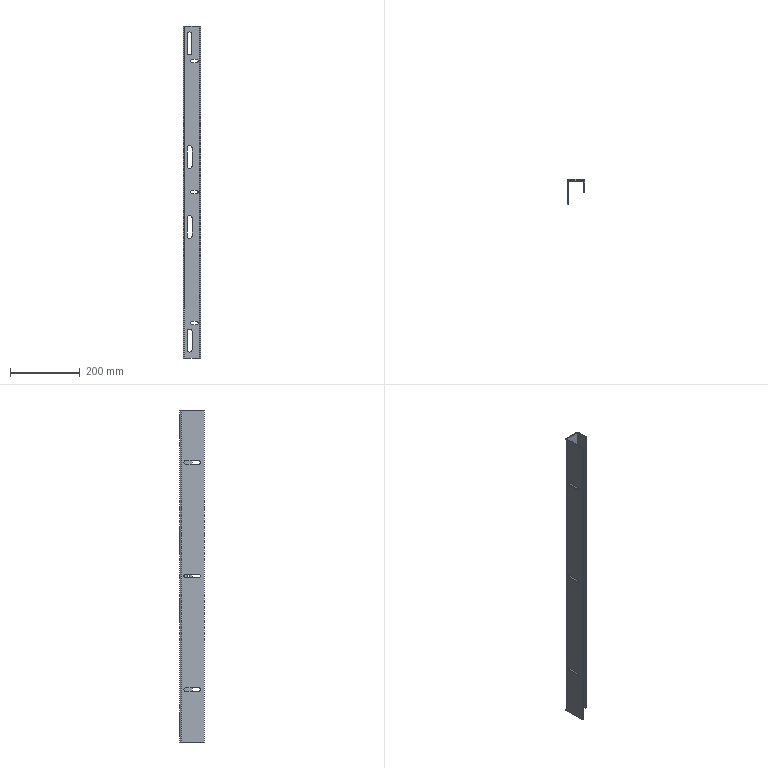Part | 1 solid | 71 faces | box 50 x 70 x 950 mm | volume 401871 mm3 | plane 38 | cylinder 33 | commonest cylinder face diameters 10 x15 14 x8 7 x6 2 x2 8 x2